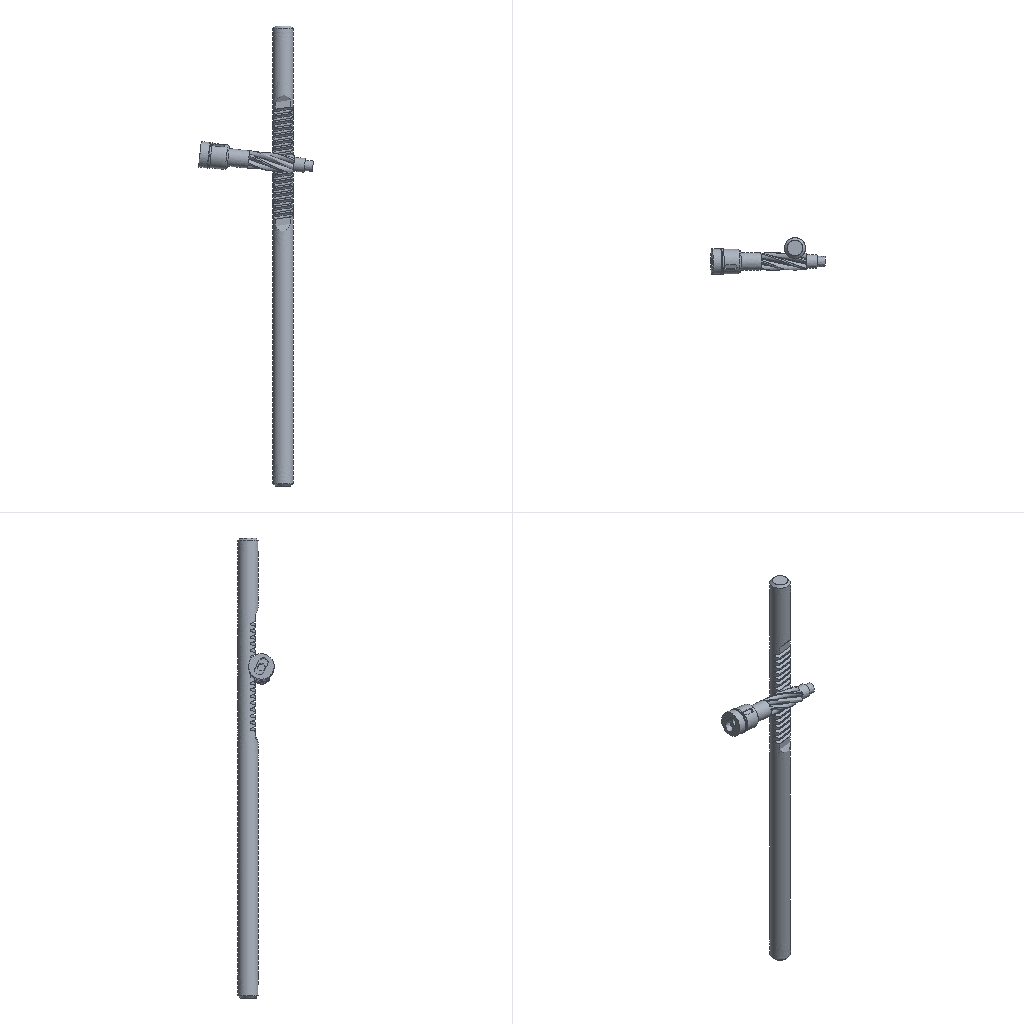Simulation study | ansys workbench
Set-up summary:
category,name,step,type,value,unit,region
solver,ansys_mapdl
solver,version,,,22.1
units,MPA,,stated
analysis,deck,,static,static
load_step,requested,,,1
analysis,nlgeom,,,False
mesh,nodes,,,276252
mesh,elements,,,175171
element_type,ANSYS 187 (type 1),,solid,62048
element_type,ANSYS 187 (type 2),,solid,101373
element_type,ANSYS 174 (type 3),,contact,1607
element_type,ANSYS 170 (type 4),,target,1607
element_type,ANSYS 174 (type 5),,contact,8536
element_type,ANSYS 170 (type 6),,target,0
load,load commands in deck,,count,3
bc,support commands in deck,,count,1
named_set,_FIXEDSU,,component
named_set,______,,component
named_set,______23,,component
material,1,,in results
material,2,,in results
check,setup vs results,,match,results also hold 0 node(s) and 1 element(s) the deck makes with ['EN']; those were not compared; 1 node(s) the solver created internally for pilot nodes (solve.out) are in the results only
Ansys APDL input file, long lists of numbers shortened:
/batch
/config,noeldb,1     ! force off writing results to database
*get,_wallstrt,active,,time,wall
! ANSYS input file written by Workbench version 2022 R1
! File used for geometry attach: F:\ansys（分析文件汇总)\齿轮齿条有限元分析\chilunchitiao.STEP
/title,wbnew--____ (B5)
! ****** Begin Custom Load Command Snippet ******
/COM, ACT Extensions:
/COM,     LSDYNA, 2021.1
/COM,
! ****** End   Custom Load Command Snippet ******
*DIM,_wb_ProjectScratch_dir,string,248
_wb_ProjectScratch_dir(1) = 'C:\Users\Administrator\AppData\Local\Temp\WB_Administrator_19260_2\_ProjectScratch\Scr30E8\'
*DIM,_wb_SolverFiles_dir,string,248
_wb_SolverFiles_dir(1) = 'C:\Users\Administrator\AppData\Local\Temp\WB_Administrator_19260_2\wbnew_files\dp0\SYS\MECH\'
*DIM,_wb_userfiles_dir,string,248
_wb_userfiles_dir(1) = 'C:\Users\Administrator\AppData\Local\Temp\WB_Administrator_19260_2\wbnew_files\user_files\'
/com,--- Data in consistent NMM units. See Solving Units in the help system for more information.
/units,MPA
/nopr
/wb,file,start              !  signify a WB generated input file
/prep7
! Turn off shape checking because checks already performed inside WB mesher.
! See help system for more information.
SHPP,OFF,,NOWARN
/nolist
etcon,set             ! allow ANSYS to choose best KEYOP's for 180x elements, resets any applicable keyopt to MAPDL defaults
/com,*********** Nodes for the whole assembly ***********
nblock,3,,303876
(1i9,3e20.9e3)
        1     1.204243006E+01    -3.351096268E+00     2.924533804E+00
! (276250 more lines like these left out)
-1
/com,*********** Nodes for all Remote Points ***********
nblock,3
(1i9,3e20.9e3)
   276252    -1.199339324E+01    -1.374958171E+01    -1.456187721E+01
-1
/wb,elem,start            !  set before creation of elements
/com,*********** Elements for Body 1 "CL.1|__________" ***********
et,1,187
eblock,19,solid,,62048
(19i9)
        1        1        1        1        0        0        0        0       10        0   101374   181590   181593   189568   184725   234881   234899   234885   234882
! (124095 more lines like these left out)
-1
/com,*********** Elements for Body 2 "11111111|__________" ***********
et,2,187
eblock,19,solid,,101373
(19i9)
        2        2        2        2        0        0        0        0       10        0        1     2021     2022    27073    25997    40839    40852    40844    40842
! (202745 more lines like these left out)
-1
/wb,elem,end               !  done creating elements
/com,*********** Send User Defined Coordinate System(s) ***********
csys,0
toffst,273.15,  ! Temperature offset from absolute zero
/com,*********** Set Reference Temperature ***********
tref,22.
/wb,mat,start              !  starting to send materials
/com,*********** Send Materials ***********
Temperature = 'TEMP' ! Temperature
MP,DENS,1,7.85e-09,	! tonne mm^-3
MP,ALPX,1,1.1e-05,	! C^-1
MP,C,1,434000000,	! mm^2 s^-2 C^-1
MP,KXX,1,60.5,	! tonne mm s^-3 C^-1
MP,RSVX,1,0.00017,	! ohm mm
MP,EX,1,200000,	! tonne s^-2 mm^-1
MP,NUXY,1,0.3,
MP,MURX,1,10000,
Temperature = 'TEMP' ! Temperature
MP,DENS,2,7.85e-09,	! tonne mm^-3
MP,ALPX,2,1.1e-05,	! C^-1
MP,C,2,434000000,	! mm^2 s^-2 C^-1
MP,KXX,2,60.5,	! tonne mm s^-3 C^-1
MP,RSVX,2,0.00017,	! ohm mm
MP,EX,2,200000,	! tonne s^-2 mm^-1
MP,NUXY,2,0.3,
MP,MURX,2,10000,
/wb,mat,end                !  done sending materials
!************************* Model Summary ********************
!CL.1|__________,	20crmnti钢,	matid,	1
!11111111|__________,	20crmnti钢,	matid,	2
!************************* End Model Summary ********************
! get the diagonal of the bounding box. Needed later for other things
*get,_xmin,node,,mnloc,x
*get,_ymin,node,,mnloc,y
*get,_zmin,node,,mnloc,z
*get,_xmax,node,,mxloc,x
*get,_ymax,node,,mxloc,y
*get,_zmax,node,,mxloc,z
_ASMDIAG=(_xmax-_xmin)*(_xmax-_xmin)+(_ymax-_ymin)*(_ymax-_ymin)+(_zmax-_zmin)*(_zmax-_zmin)
_ASMDIAG=SQRT(_ASMDIAG)
/wb,contact,start          !  starting to send contact
/com,*********** Create Contact "接触区域" ***********
/com,            Real Constant Set For Above Contact Is 4 & 3
*set,tid,4
*set,cid,3
r,tid
r,cid
et,tid,170
et,cid,174
eblock,10,,,850
(15i9)
   219391        4        4        4        0   177116   181618   178189   178189   211102   216955   178189   211100
! (849 more lines like these left out)
-1
eblock,10,,,850
(15i9)
   220241        3        3        3        0   177116   181618   178189   178189   211102   216955   178189   211100
! (849 more lines like these left out)
-1
eblock,10,,,757
(15i9)
   221091        3        4        3        0       26    18087    18086    18086    27260   129194    18086    27259
! (756 more lines like these left out)
-1
eblock,10,,,757
(15i9)
   221848        4        3        4        0       26    18087    18086    18086    27260   129194    18086    27259
! (756 more lines like these left out)
-1
keyo,cid,8,2               ! auto create asymmetric contact (from Program Controlled setting)
keyo,cid,10,0              ! adjust contact stiffness each NR iteration (from Program Controlled setting)
keyo,cid,12,5              ! bonded always
keyo,cid,18,1              ! small sliding turned on by application
keyo,cid,2,0               ! augmented Lagrange (from Program Controlled setting)
keyo,cid,4,0               ! on Gauss point (from Program Controlled setting)
keyo,cid,9,1               ! ignore initial gaps/penetration
keyo,cid,7,0               ! No Prediction
rmod,tid,3,10.      ! FKN
rmod,tid,5,0.       ! ICONT
rmod,tid,6,0.       ! PINB
rmod,tid,10,0.      ! CNOF
rmod,tid,12,0.      ! FKT
rmod,tid,36,29      ! WB DSID
rmod,cid,3,10.      ! FKN
rmod,cid,5,0.       ! ICONT
rmod,cid,6,0.       ! PINB
rmod,cid,10,0.      ! CNOF
rmod,cid,12,0.      ! FKT
rmod,cid,36,29      ! WB DSID
nsel,all
esel,all
/wb,contact,end            !  done creating contacts
/com,*********** Send Named Selection as Node Component ***********
CMBLOCK,______  ,NODE,    18698
(8i10)
      2485      2502      2504      2505      2506      2507      2508      2509
! (2337 more lines like these left out)
/com,*********** Send Named Selection as Node Component ***********
CMBLOCK,______23,NODE,    42992
(8i10)
         1         2         3         4         5         6         7         8
! (5373 more lines like these left out)
/golist
/wb,load,start             !  starting to send loads
/com,*********** Fixed Supports ***********
CMBLOCK,_FIXEDSU,NODE,     3412
(8i10)
      2485      2502      2504      2505      2506      2507      2508      2509
! (426 more lines like these left out)
cmsel,s,_FIXEDSU
d,all,all
nsel,all
/com,*********** Create Remote Point "内部远程点" ***********
! -------- Remote Point Used by "力矩" --------
*set,tid,6
*set,cid,5
et,cid,174
et,tid,170
keyo,tid,2,1               ! Don't fix the pilot node
keyo,tid,4,111111
keyo,cid,12,5              ! Bonded Contact
keyo,cid,4,1               ! Deformable RBE3 style load
keyo,cid,2,2               ! MPC style contact
eblock,10,,,8536
(15i9)
   222605        5        5        5        0   181188   181357   181241   181241   232957   233318   181241   232955
! (8535 more lines like these left out)
-1
*set,_npilot,276252
_npilot42=_npilot
type,tid
mat ,cid
real,cid
tshape,pilo
en,231141,_npilot
tshape
/com,*********** Construct Moment Using Remote Attachment ***********
/gst,on,on
fini
*get,_numnode,node,0,count
*get,_numelem,elem,0,count
*get, _MAXELEMNUM, elem, 0, NUM, MAX
*get, _MAXNODENUM, node, 0, NUM, MAX
*get, _MAXELEMTYPE, etyp, 0, NUM, MAX
*get, _MAXREALCONST, real, 0, NUM, MAX
/go
/wb,load,end               !  done creating loads
/com,--- Number of total nodes = %_numnode%
/com,--- Number of contact elements = 11750
/com,--- Number of spring elements = 0
/com,--- Number of bearing elements = 0
/com,--- Number of solid elements = 163421
/com,--- Number of condensed parts = 0
/com,--- Number of total elements = %_numelem%
*get,_wallbsol,active,,time,wall
/com,****************************************************************************
/com,*************************    SOLUTION       ********************************
/com,****************************************************************************
/solu
antype,0                   ! static analysis
_thickRatio=  1     ! Ratio of thick parts in the model
eqsl,pcg,1e-8,,,,,,1
cntr,print,1               ! print out contact info and also make no initial contact an error
dmpoption,emat,no             ! Don't combine emat file for DANSYS
dmpoption,esav,no             ! Don't combine esav file for DANSYS
nldiag,cont,iter           ! print out contact info each equilibrium iteration
rescontrol,,none                 ! Do not keep any restart files
/com,****************************************************
/com,******************* SOLVE FOR LS 1 OF 1 ****************
nsel,s,node,,276252
f,all,mx,904400.
f,all,my,0.
f,all,mz,0.
nsel,all
/nopr
/gopr
nsub,1,1,1
time,1.
outres,erase
outres,all,none
outres,nsol,all,
outres,rsol,all
outres,eangl,all
outres,etmp,all
outres,veng,all
outres,strs,all,
outres,epel,all,
outres,eppl,all,
outres,cont,all,
! *********** WB SOLVE COMMAND ***********
! check interactive state
*get,ANSINTER_,active,,int
*if,ANSINTER_,ne,0,then
/eof
*endif
solve
/com *************** Write FE CONNECTORS *********
CEWRITE,file,ce,,INTE
/com,****************************************************
/com,*************** FINISHED SOLVE FOR LS 1 *************
*get,_wallasol,active,,time,wall
/nopr
*get,_numnode,node,0,count
*get,_numelem,elem,0,count
*get, _MAXELEMNUM, elem, 0, NUM, MAX
*get, _MAXNODENUM, node, 0, NUM, MAX,,,INTERNAL
*get, _MAXELEMTYPE, etyp, 0, NUM, MAX
*get, _MAXREALCONST, real, 0, NUM, MAX
/gopr
*get,_PCGITER,active,,solu,cgiter
/post1
xmlo,ENCODING,ISO-8859-1
xmlo,parm
/xml,parm,xml
fini
/gopr
*get,_walldone,active,,time,wall
_preptime=(_wallbsol-_wallstrt)*3600
_solvtime=(_wallasol-_wallbsol)*3600
_posttime=(_walldone-_wallasol)*3600
_totaltim=(_walldone-_wallstrt)*3600
*get,_dlbratio,active,0,solu,dlbr
*get,_combtime,active,0,solu,comb
*get,_ssmode,active,0,solu,ssmm
*get,_ndofs,active,0,solu,ndof
*get,_sol_end_time,active,0,set,time
*if,_sol_end_time,eq,1.,then
/fclean				!clean distributed files
*endif
/com,--- Total number of nodes = %_numnode%
/com,--- Total number of elements = %_numelem%
/com,--- Element load balance ratio = %_dlbratio%
/com,--- Time to combine distributed files = %_combtime%
/com,--- Sparse memory mode = %_ssmode%
/com,--- Number of DOF = %_ndofs%
/wb,file,end               ! done with WB generated input
Results summary:
result,analysis,,,static
result,last_loadstep,,,1
result,primary field,,,displacement
result,reaction total,1,FX,1e-06,N
result,reaction total,1,FY,-1e-06,N
result,reaction total,1,FZ,-3e-06,N
result,mass,,,0.002402,"NMM: mm, ton, N, s, mV, mA, degC"